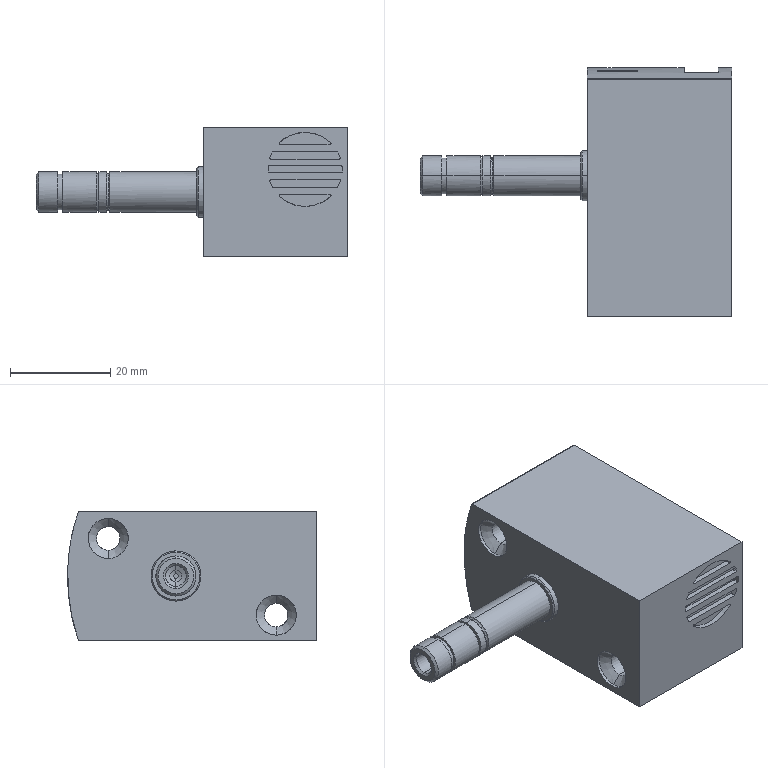Part | SolidWorks | features BaseBody 1 | 1 solid | 141 faces | box 62.1 x 49.6 x 25.9 mm | volume 36554 mm3 | plane 63 | cylinder 58 | cone 16 | torus 4 | commonest cylinder face diameters 0.4 x18 8 x12 14.8 x8 4.7 x4 0.9 x2 2.4 x2